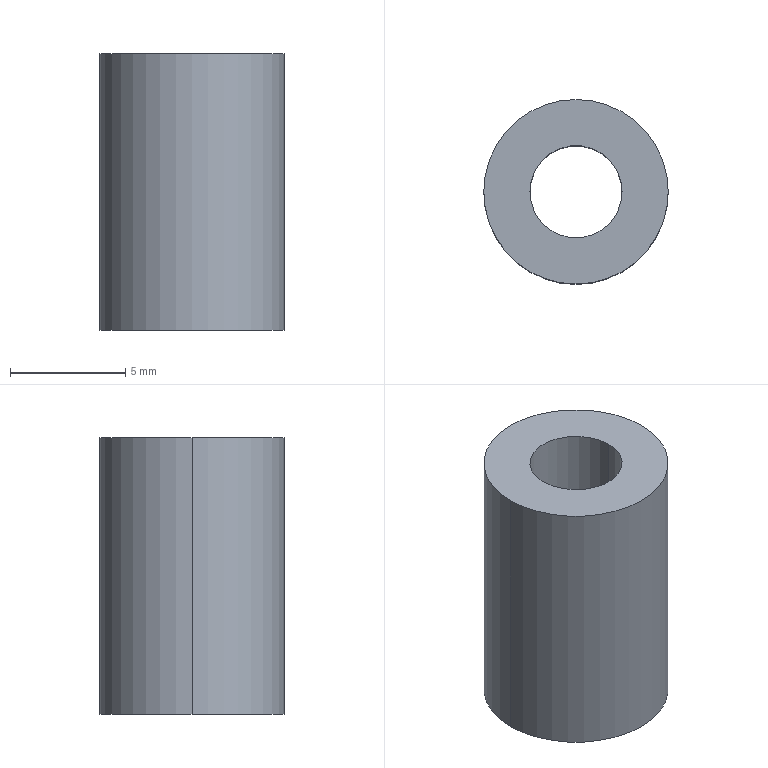Part | SolidWorks | features BaseBody 1 | 1 solid | 6 faces | box 8 x 8 x 12 mm | volume 452.389 mm3 | cylinder 4 | plane 2 | commonest cylinder face diameters 4 x2 8 x2
STEP:
#1=CARTESIAN_POINT('',(-4.,0.,6.));
#2=VERTEX_POINT('',#1);
#3=CARTESIAN_POINT('',(4.,0.,6.));
#4=VERTEX_POINT('',#3);
#5=CARTESIAN_POINT('',(0.,0.,6.));
#6=DIRECTION('',(0.,0.,-1.));
#7=DIRECTION('',(-1.,0.,0.));
#8=AXIS2_PLACEMENT_3D('',#5,#6,#7);
#9=CIRCLE('',#8,4.);
#10=EDGE_CURVE('',#2,#4,#9,.T.);
#11=ORIENTED_EDGE('',*,*,#10,.T.);
#12=CARTESIAN_POINT('',(4.,0.,-6.));
#13=VERTEX_POINT('',#12);
#14=CARTESIAN_POINT('',(4.,0.,6.));
#15=DIRECTION('',(0.,0.,-1.));
#16=VECTOR('',#15,1000.);
#17=LINE('',#14,#16);
#18=EDGE_CURVE('',#4,#13,#17,.T.);
#19=ORIENTED_EDGE('',*,*,#18,.T.);
#20=CARTESIAN_POINT('',(-4.,0.,-6.));
#21=VERTEX_POINT('',#20);
#22=CARTESIAN_POINT('',(0.,0.,-6.));
#23=DIRECTION('',(0.,0.,1.));
#24=DIRECTION('',(-1.,0.,0.));
#25=AXIS2_PLACEMENT_3D('',#22,#23,#24);
#26=CIRCLE('',#25,4.);
#27=EDGE_CURVE('',#13,#21,#26,.T.);
#28=ORIENTED_EDGE('',*,*,#27,.T.);
#29=CARTESIAN_POINT('',(-4.,0.,6.));
#30=DIRECTION('',(0.,0.,-1.));
#31=VECTOR('',#30,1000.);
#32=LINE('',#29,#31);
#33=EDGE_CURVE('',#2,#21,#32,.T.);
#34=ORIENTED_EDGE('',*,*,#33,.F.);
#35=EDGE_LOOP('',(#11,#19,#28,#34));
#36=FACE_OUTER_BOUND('',#35,.T.);
#37=CARTESIAN_POINT('',(0.,0.,6.));
#38=DIRECTION('',(0.,0.,-1.));
#39=DIRECTION('',(-1.,0.,0.));
#40=AXIS2_PLACEMENT_3D('',#37,#38,#39);
#41=CYLINDRICAL_SURFACE('',#40,4.);
#42=ADVANCED_FACE('',(#36),#41,.T.);
#43=CARTESIAN_POINT('',(2.,0.,6.));
#44=VERTEX_POINT('',#43);
#45=CARTESIAN_POINT('',(-2.,0.,6.));
#46=VERTEX_POINT('',#45);
#47=CARTESIAN_POINT('',(0.,0.,6.));
#48=DIRECTION('',(0.,0.,-1.));
#49=DIRECTION('',(-1.,0.,0.));
#50=AXIS2_PLACEMENT_3D('',#47,#48,#49);
#51=CIRCLE('',#50,2.);
#52=EDGE_CURVE('',#44,#46,#51,.T.);
#53=ORIENTED_EDGE('',*,*,#52,.F.);
#54=CARTESIAN_POINT('',(2.,0.,-6.));
#55=VERTEX_POINT('',#54);
#56=CARTESIAN_POINT('',(2.,0.,6.));
#57=DIRECTION('',(0.,0.,-1.));
#58=VECTOR('',#57,1000.);
#59=LINE('',#56,#58);
#60=EDGE_CURVE('',#44,#55,#59,.T.);
#61=ORIENTED_EDGE('',*,*,#60,.T.);
#62=CARTESIAN_POINT('',(-2.,0.,-6.));
#63=VERTEX_POINT('',#62);
#64=CARTESIAN_POINT('',(0.,0.,-6.));
#65=DIRECTION('',(0.,0.,-1.));
#66=DIRECTION('',(-1.,0.,0.));
#67=AXIS2_PLACEMENT_3D('',#64,#65,#66);
#68=CIRCLE('',#67,2.);
#69=EDGE_CURVE('',#55,#63,#68,.T.);
#70=ORIENTED_EDGE('',*,*,#69,.T.);
#71=CARTESIAN_POINT('',(-2.,0.,6.));
#72=DIRECTION('',(0.,0.,-1.));
#73=VECTOR('',#72,1000.);
#74=LINE('',#71,#73);
#75=EDGE_CURVE('',#46,#63,#74,.T.);
#76=ORIENTED_EDGE('',*,*,#75,.F.);
#77=EDGE_LOOP('',(#53,#61,#70,#76));
#78=FACE_OUTER_BOUND('',#77,.T.);
#79=CARTESIAN_POINT('',(0.,0.,6.));
#80=DIRECTION('',(0.,0.,-1.));
#81=DIRECTION('',(-1.,0.,0.));
#82=AXIS2_PLACEMENT_3D('',#79,#80,#81);
#83=CYLINDRICAL_SURFACE('',#82,2.);
#84=ADVANCED_FACE('',(#78),#83,.F.);
#85=ORIENTED_EDGE('',*,*,#18,.F.);
#86=CARTESIAN_POINT('',(0.,0.,6.));
#87=DIRECTION('',(0.,0.,-1.));
#88=DIRECTION('',(-1.,0.,0.));
#89=AXIS2_PLACEMENT_3D('',#86,#87,#88);
#90=CIRCLE('',#89,4.);
#91=EDGE_CURVE('',#4,#2,#90,.T.);
#92=ORIENTED_EDGE('',*,*,#91,.T.);
#93=ORIENTED_EDGE('',*,*,#33,.T.);
#94=CARTESIAN_POINT('',(0.,0.,-6.));
#95=DIRECTION('',(0.,0.,1.));
#96=DIRECTION('',(-1.,0.,0.));
#97=AXIS2_PLACEMENT_3D('',#94,#95,#96);
#98=CIRCLE('',#97,4.);
#99=EDGE_CURVE('',#21,#13,#98,.T.);
#100=ORIENTED_EDGE('',*,*,#99,.T.);
#101=EDGE_LOOP('',(#85,#92,#93,#100));
#102=FACE_OUTER_BOUND('',#101,.T.);
#103=CARTESIAN_POINT('',(0.,0.,6.));
#104=DIRECTION('',(0.,0.,-1.));
#105=DIRECTION('',(-1.,0.,0.));
#106=AXIS2_PLACEMENT_3D('',#103,#104,#105);
#107=CYLINDRICAL_SURFACE('',#106,4.);
#108=ADVANCED_FACE('',(#102),#107,.T.);
#109=CARTESIAN_POINT('',(0.,0.,-6.));
#110=DIRECTION('',(0.,0.,-1.));
#111=DIRECTION('',(-1.,0.,0.));
#112=AXIS2_PLACEMENT_3D('',#109,#110,#111);
#113=CIRCLE('',#112,2.);
#114=EDGE_CURVE('',#63,#55,#113,.T.);
#115=ORIENTED_EDGE('',*,*,#114,.F.);
#116=ORIENTED_EDGE('',*,*,#69,.F.);
#117=EDGE_LOOP('',(#115,#116));
#118=FACE_BOUND('',#117,.T.);
#119=ORIENTED_EDGE('',*,*,#99,.F.);
#120=ORIENTED_EDGE('',*,*,#27,.F.);
#121=EDGE_LOOP('',(#119,#120));
#122=FACE_OUTER_BOUND('',#121,.T.);
#123=CARTESIAN_POINT('',(0.,0.,-6.));
#124=DIRECTION('',(0.,0.,1.));
#125=DIRECTION('',(1.,0.,0.));
#126=AXIS2_PLACEMENT_3D('',#123,#124,#125);
#127=PLANE('',#126);
#128=ADVANCED_FACE('',(#118,#122),#127,.F.);
#129=CARTESIAN_POINT('',(0.,0.,6.));
#130=DIRECTION('',(0.,0.,-1.));
#131=DIRECTION('',(-1.,0.,0.));
#132=AXIS2_PLACEMENT_3D('',#129,#130,#131);
#133=CIRCLE('',#132,2.);
#134=EDGE_CURVE('',#46,#44,#133,.T.);
#135=ORIENTED_EDGE('',*,*,#134,.T.);
#136=ORIENTED_EDGE('',*,*,#52,.T.);
#137=EDGE_LOOP('',(#135,#136));
#138=FACE_BOUND('',#137,.T.);
#139=ORIENTED_EDGE('',*,*,#10,.F.);
#140=ORIENTED_EDGE('',*,*,#91,.F.);
#141=EDGE_LOOP('',(#139,#140));
#142=FACE_OUTER_BOUND('',#141,.T.);
#143=CARTESIAN_POINT('',(0.,0.,6.));
#144=DIRECTION('',(0.,0.,1.));
#145=DIRECTION('',(1.,0.,0.));
#146=AXIS2_PLACEMENT_3D('',#143,#144,#145);
#147=PLANE('',#146);
#148=ADVANCED_FACE('',(#138,#142),#147,.T.);
#149=ORIENTED_EDGE('',*,*,#60,.F.);
#150=ORIENTED_EDGE('',*,*,#134,.F.);
#151=ORIENTED_EDGE('',*,*,#75,.T.);
#152=ORIENTED_EDGE('',*,*,#114,.T.);
#153=EDGE_LOOP('',(#149,#150,#151,#152));
#154=FACE_OUTER_BOUND('',#153,.T.);
#155=CARTESIAN_POINT('',(0.,0.,6.));
#156=DIRECTION('',(0.,0.,-1.));
#157=DIRECTION('',(-1.,0.,0.));
#158=AXIS2_PLACEMENT_3D('',#155,#156,#157);
#159=CYLINDRICAL_SURFACE('',#158,2.);
#160=ADVANCED_FACE('',(#154),#159,.F.);
#161=CLOSED_SHELL('',(#42,#84,#108,#128,#148,#160));
#162=MANIFOLD_SOLID_BREP('',#161);
#163=CARTESIAN_POINT('',(0.,0.,0.));
#164=DIRECTION('',(0.,0.,1.));
#165=DIRECTION('',(1.,0.,0.));
#166=AXIS2_PLACEMENT_3D('',#163,#164,#165);
#167=(LENGTH_UNIT()NAMED_UNIT(*)SI_UNIT(.MILLI.,.METRE.));
#168=UNCERTAINTY_MEASURE_WITH_UNIT(LENGTH_MEASURE(0.00001),#167,'','');
#169=(NAMED_UNIT(*)PLANE_ANGLE_UNIT()SI_UNIT($,.RADIAN.));
#170=(NAMED_UNIT(*)SI_UNIT($,.STERADIAN.)SOLID_ANGLE_UNIT());
#171=(GEOMETRIC_REPRESENTATION_CONTEXT(3)GLOBAL_UNCERTAINTY_ASSIGNED_CONTEXT((#168))GLOBAL_UNIT_ASSIGNED_CONTEXT((#167,#169,#170))REPRESENTATION_CONTEXT('',''));
#172=ADVANCED_BREP_SHAPE_REPRESENTATION('',(#162,#166),#171);